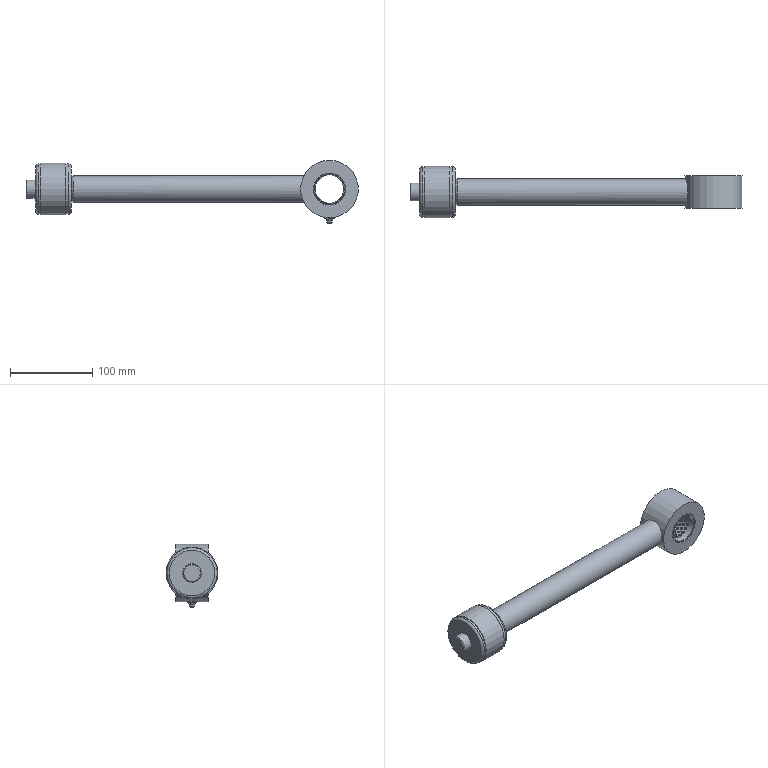Part | STEP file | HL7YG-5.59.024_抓具油缸(活塞杆)--000.002--20240512 | 7 solids | 178 faces | box 404.5 x 63 x 77.2 mm | volume 476577 mm3 | spline 100 | plane 37 | cylinder 27 | cone 10 | torus 3 | sphere 1 | commonest cylinder face diameters 24 x4 58.4 x4 30 x2 39 x2 47 x2 61.5 x2